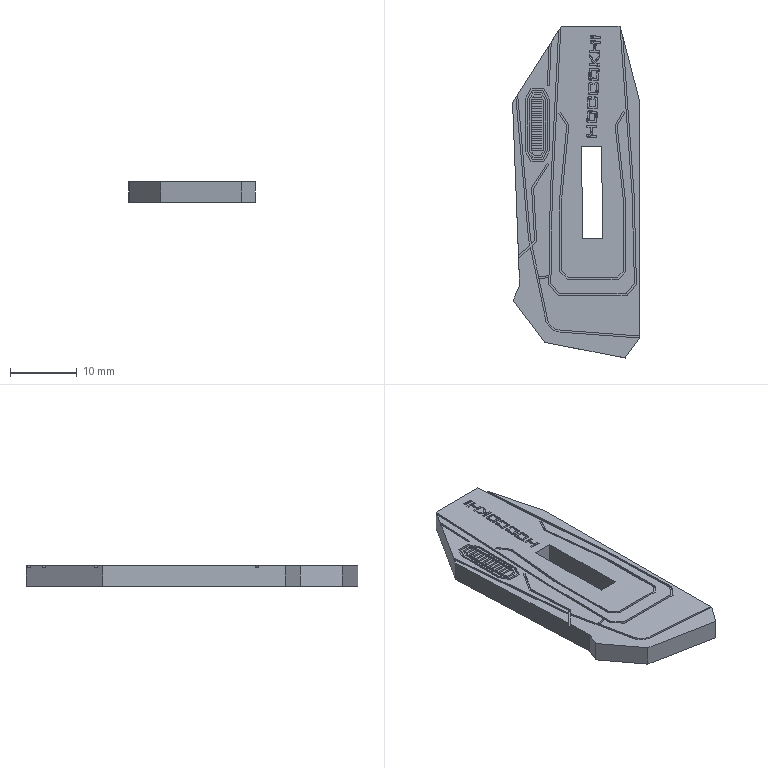Part | SolidWorks | features BaseBody 1 | 1 solid | 286 faces | box 18.994 x 49.692 x 3 mm | volume 2324 mm3 | plane 260 | spline 26